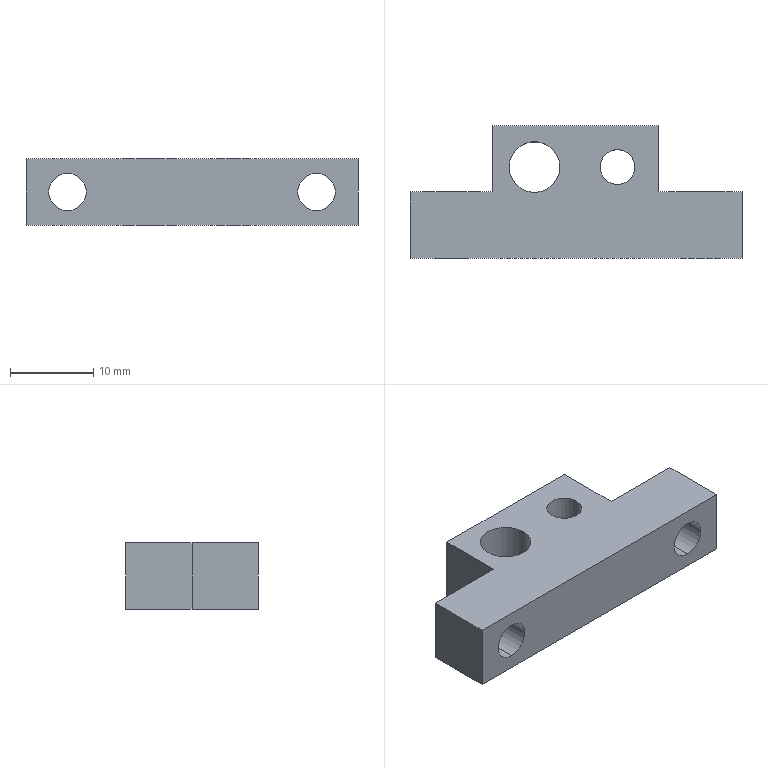Part | STEP file | Harpoon shift buffer fixing seat | 1 solid | 24 faces | box 40 x 16 x 8 mm | volume 2986 mm3 | cylinder 12 | plane 12 | commonest cylinder face diameters 4.5 x4 7.5 x4 4.2 x2 6.1 x2